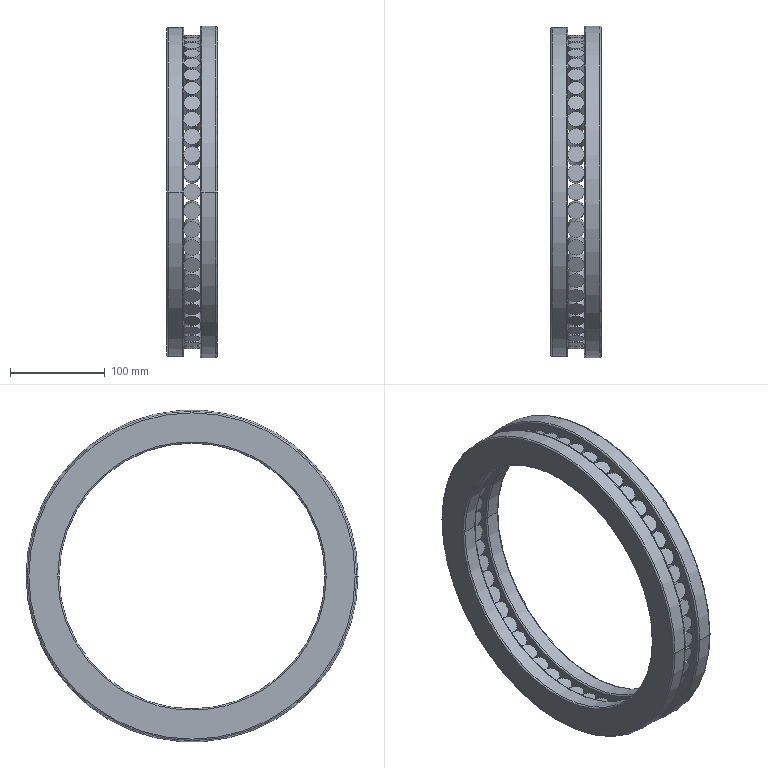Part | SolidWorks | features Revolution 3, CirPattern 1, Fillet 1 | 1 solid | 288 faces | box 53 x 350 x 350 mm | volume 1385597 mm3 | cylinder 164 | plane 108 | torus 16 | commonest cylinder face diameters 17.867 x156 280 x2 283 x2 347 x2 350 x2